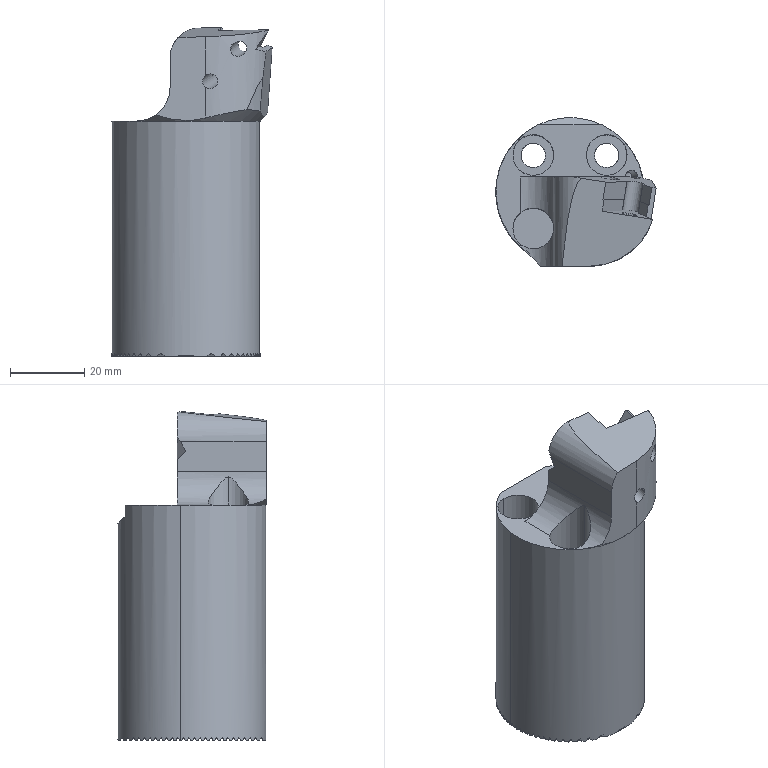Part | 1 solid | 198 faces | volume 69363 mm3 | plane 163 | cylinder 33 | cone 2 | commonest cylinder face diameters 11 x6 4 x5 6.6 x4 1.5 x2 2.9 x2 3.3 x2